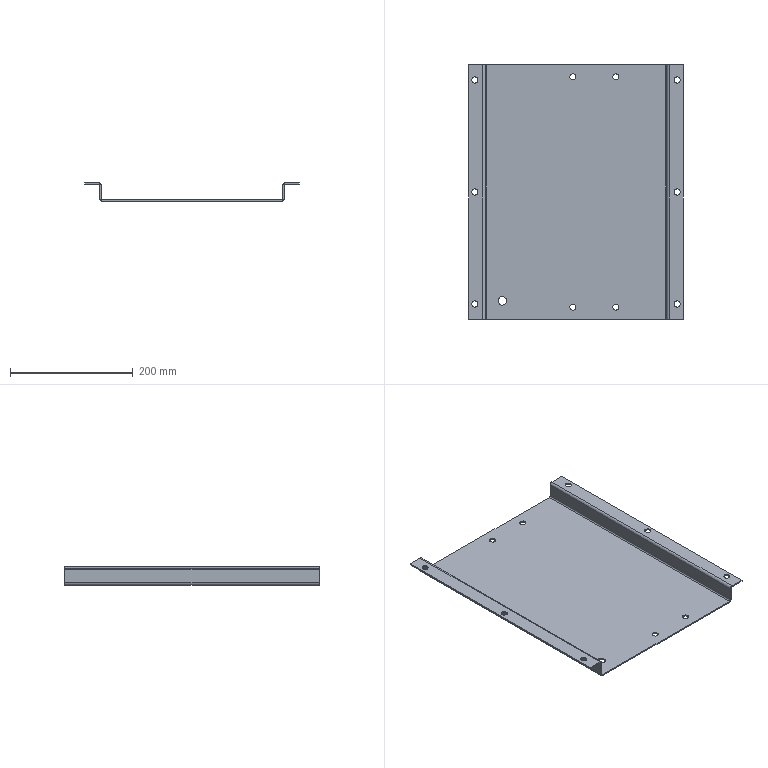Part | SolidWorks | features EdgeFlange 2, ICE 2, FlatPattern 1, SMBaseFlange 1, SheetMetal 1 | 1 solid | 60 faces | box 350 x 415 x 30 mm | volume 330826 mm3 | cylinder 30 | plane 30 | commonest cylinder face diameters 10 x20 4 x4 8 x4 14 x2